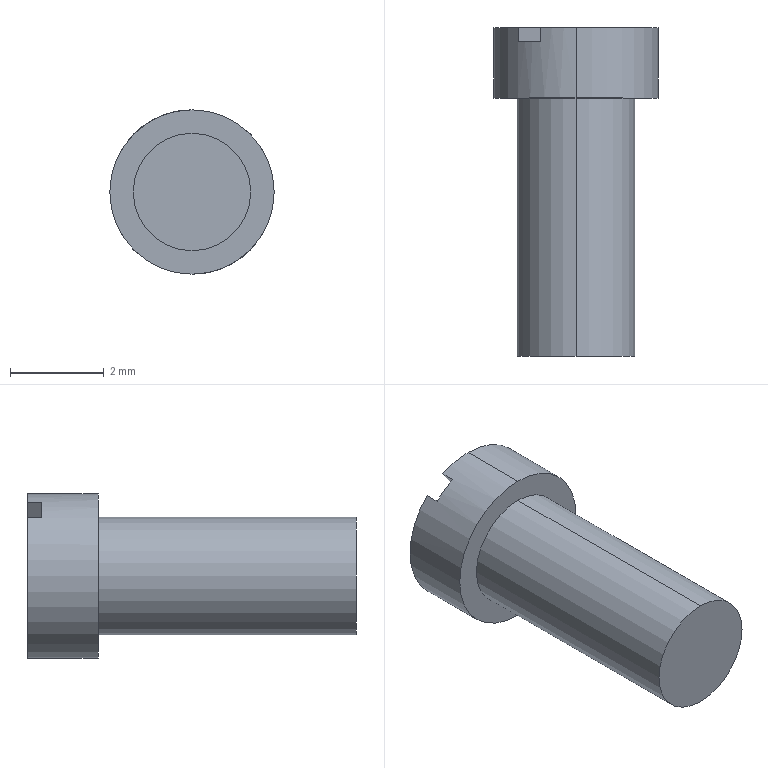Part | SolidWorks | features Cut 1, Extrusion 1, ICE 1 | 1 solid | 11 faces | box 3.5 x 7 x 3.5 mm | volume 40.83 mm3 | plane 7 | cylinder 4 | commonest cylinder face diameters 2.5 x2 3.5 x2
STEP:
#1=CARTESIAN_POINT('',(0.,7.,1.75));
#2=VERTEX_POINT('',#1);
#3=CARTESIAN_POINT('',(1.233,7.,-1.242));
#4=VERTEX_POINT('',#3);
#5=CARTESIAN_POINT('',(0.,7.,0.));
#6=DIRECTION('',(0.,1.,0.));
#7=DIRECTION('',(0.,0.,1.));
#8=AXIS2_PLACEMENT_3D('',#5,#6,#7);
#9=CIRCLE('',#8,1.75);
#10=EDGE_CURVE('',#2,#4,#9,.T.);
#11=ORIENTED_EDGE('',*,*,#10,.F.);
#12=CARTESIAN_POINT('',(0.,5.5,1.75));
#13=VERTEX_POINT('',#12);
#14=CARTESIAN_POINT('',(0.,7.,1.75));
#15=DIRECTION('',(0.,-1.,0.));
#16=VECTOR('',#15,1000.);
#17=LINE('',#14,#16);
#18=EDGE_CURVE('',#2,#13,#17,.T.);
#19=ORIENTED_EDGE('',*,*,#18,.T.);
#20=CARTESIAN_POINT('',(0.,5.5,-1.75));
#21=VERTEX_POINT('',#20);
#22=CARTESIAN_POINT('',(0.,5.5,0.));
#23=DIRECTION('',(0.,1.,0.));
#24=DIRECTION('',(0.,0.,1.));
#25=AXIS2_PLACEMENT_3D('',#22,#23,#24);
#26=CIRCLE('',#25,1.75);
#27=EDGE_CURVE('',#13,#21,#26,.T.);
#28=ORIENTED_EDGE('',*,*,#27,.T.);
#29=CARTESIAN_POINT('',(0.,7.,-1.75));
#30=VERTEX_POINT('',#29);
#31=CARTESIAN_POINT('',(0.,7.,-1.75));
#32=DIRECTION('',(0.,-1.,0.));
#33=VECTOR('',#32,1000.);
#34=LINE('',#31,#33);
#35=EDGE_CURVE('',#30,#21,#34,.T.);
#36=ORIENTED_EDGE('',*,*,#35,.F.);
#37=CARTESIAN_POINT('',(0.7649,7.,-1.574));
#38=VERTEX_POINT('',#37);
#39=CARTESIAN_POINT('',(0.,7.,0.));
#40=DIRECTION('',(0.,1.,0.));
#41=DIRECTION('',(0.,0.,1.));
#42=AXIS2_PLACEMENT_3D('',#39,#40,#41);
#43=CIRCLE('',#42,1.75);
#44=EDGE_CURVE('',#38,#30,#43,.T.);
#45=ORIENTED_EDGE('',*,*,#44,.F.);
#46=CARTESIAN_POINT('',(0.7649,6.7,-1.574));
#47=VERTEX_POINT('',#46);
#48=CARTESIAN_POINT('',(0.7649,7.,-1.574));
#49=DIRECTION('',(0.,-1.,0.));
#50=VECTOR('',#49,1000.);
#51=LINE('',#48,#50);
#52=EDGE_CURVE('',#38,#47,#51,.T.);
#53=ORIENTED_EDGE('',*,*,#52,.T.);
#54=CARTESIAN_POINT('',(1.233,6.7,-1.242));
#55=VERTEX_POINT('',#54);
#56=CARTESIAN_POINT('',(0.,6.7,0.));
#57=DIRECTION('',(0.,1.,0.));
#58=DIRECTION('',(0.,0.,1.));
#59=AXIS2_PLACEMENT_3D('',#56,#57,#58);
#60=CIRCLE('',#59,1.75);
#61=EDGE_CURVE('',#55,#47,#60,.T.);
#62=ORIENTED_EDGE('',*,*,#61,.F.);
#63=CARTESIAN_POINT('',(1.233,7.,-1.242));
#64=DIRECTION('',(0.,1.,0.));
#65=VECTOR('',#64,1000.);
#66=LINE('',#63,#65);
#67=EDGE_CURVE('',#55,#4,#66,.T.);
#68=ORIENTED_EDGE('',*,*,#67,.T.);
#69=EDGE_LOOP('',(#11,#19,#28,#36,#45,#53,#62,#68));
#70=FACE_OUTER_BOUND('',#69,.T.);
#71=CARTESIAN_POINT('',(0.,7.,0.));
#72=DIRECTION('',(0.,-1.,0.));
#73=DIRECTION('',(0.,0.,-1.));
#74=AXIS2_PLACEMENT_3D('',#71,#72,#73);
#75=CYLINDRICAL_SURFACE('',#74,1.75);
#76=ADVANCED_FACE('',(#70),#75,.T.);
#77=CARTESIAN_POINT('',(0.,5.5,1.25));
#78=VERTEX_POINT('',#77);
#79=CARTESIAN_POINT('',(0.,5.5,-1.25));
#80=VERTEX_POINT('',#79);
#81=CARTESIAN_POINT('',(0.,5.5,0.));
#82=DIRECTION('',(0.,1.,0.));
#83=DIRECTION('',(0.,0.,1.));
#84=AXIS2_PLACEMENT_3D('',#81,#82,#83);
#85=CIRCLE('',#84,1.25);
#86=EDGE_CURVE('',#78,#80,#85,.T.);
#87=ORIENTED_EDGE('',*,*,#86,.F.);
#88=CARTESIAN_POINT('',(0.,0.,1.25));
#89=VERTEX_POINT('',#88);
#90=CARTESIAN_POINT('',(0.,5.5,1.25));
#91=DIRECTION('',(0.,-1.,0.));
#92=VECTOR('',#91,1000.);
#93=LINE('',#90,#92);
#94=EDGE_CURVE('',#78,#89,#93,.T.);
#95=ORIENTED_EDGE('',*,*,#94,.T.);
#96=CARTESIAN_POINT('',(0.,0.,-1.25));
#97=VERTEX_POINT('',#96);
#98=CARTESIAN_POINT('',(0.,0.,0.));
#99=DIRECTION('',(0.,1.,0.));
#100=DIRECTION('',(0.,0.,1.));
#101=AXIS2_PLACEMENT_3D('',#98,#99,#100);
#102=CIRCLE('',#101,1.25);
#103=EDGE_CURVE('',#89,#97,#102,.T.);
#104=ORIENTED_EDGE('',*,*,#103,.T.);
#105=CARTESIAN_POINT('',(0.,5.5,-1.25));
#106=DIRECTION('',(0.,-1.,0.));
#107=VECTOR('',#106,1000.);
#108=LINE('',#105,#107);
#109=EDGE_CURVE('',#80,#97,#108,.T.);
#110=ORIENTED_EDGE('',*,*,#109,.F.);
#111=EDGE_LOOP('',(#87,#95,#104,#110));
#112=FACE_OUTER_BOUND('',#111,.T.);
#113=CARTESIAN_POINT('',(0.,5.5,0.));
#114=DIRECTION('',(0.,-1.,0.));
#115=DIRECTION('',(0.,0.,-1.));
#116=AXIS2_PLACEMENT_3D('',#113,#114,#115);
#117=CYLINDRICAL_SURFACE('',#116,1.25);
#118=ADVANCED_FACE('',(#112),#117,.T.);
#119=CARTESIAN_POINT('',(-1.233,7.,1.242));
#120=VERTEX_POINT('',#119);
#121=CARTESIAN_POINT('',(-0.2341,7.,-0.1661));
#122=DIRECTION('',(-0.5787,0.,0.8155));
#123=VECTOR('',#122,1000.);
#124=LINE('',#121,#123);
#125=EDGE_CURVE('',#38,#120,#124,.T.);
#126=ORIENTED_EDGE('',*,*,#125,.F.);
#127=ORIENTED_EDGE('',*,*,#44,.T.);
#128=CARTESIAN_POINT('',(0.,7.,0.));
#129=DIRECTION('',(0.,1.,0.));
#130=DIRECTION('',(0.,0.,1.));
#131=AXIS2_PLACEMENT_3D('',#128,#129,#130);
#132=CIRCLE('',#131,1.75);
#133=EDGE_CURVE('',#30,#120,#132,.T.);
#134=ORIENTED_EDGE('',*,*,#133,.T.);
#135=EDGE_LOOP('',(#126,#127,#134));
#136=FACE_OUTER_BOUND('',#135,.T.);
#137=CARTESIAN_POINT('',(0.,7.,0.));
#138=DIRECTION('',(0.,1.,0.));
#139=DIRECTION('',(0.,0.,1.));
#140=AXIS2_PLACEMENT_3D('',#137,#138,#139);
#141=PLANE('',#140);
#142=ADVANCED_FACE('',(#136),#141,.T.);
#143=ORIENTED_EDGE('',*,*,#94,.F.);
#144=CARTESIAN_POINT('',(0.,5.5,0.));
#145=DIRECTION('',(0.,1.,0.));
#146=DIRECTION('',(0.,0.,1.));
#147=AXIS2_PLACEMENT_3D('',#144,#145,#146);
#148=CIRCLE('',#147,1.25);
#149=EDGE_CURVE('',#80,#78,#148,.T.);
#150=ORIENTED_EDGE('',*,*,#149,.F.);
#151=ORIENTED_EDGE('',*,*,#109,.T.);
#152=CARTESIAN_POINT('',(0.,0.,0.));
#153=DIRECTION('',(0.,1.,0.));
#154=DIRECTION('',(0.,0.,1.));
#155=AXIS2_PLACEMENT_3D('',#152,#153,#154);
#156=CIRCLE('',#155,1.25);
#157=EDGE_CURVE('',#97,#89,#156,.T.);
#158=ORIENTED_EDGE('',*,*,#157,.T.);
#159=EDGE_LOOP('',(#143,#150,#151,#158));
#160=FACE_OUTER_BOUND('',#159,.T.);
#161=CARTESIAN_POINT('',(0.,5.5,0.));
#162=DIRECTION('',(0.,-1.,0.));
#163=DIRECTION('',(0.,0.,-1.));
#164=AXIS2_PLACEMENT_3D('',#161,#162,#163);
#165=CYLINDRICAL_SURFACE('',#164,1.25);
#166=ADVANCED_FACE('',(#160),#165,.T.);
#167=ORIENTED_EDGE('',*,*,#157,.F.);
#168=ORIENTED_EDGE('',*,*,#103,.F.);
#169=EDGE_LOOP('',(#167,#168));
#170=FACE_OUTER_BOUND('',#169,.T.);
#171=CARTESIAN_POINT('',(0.,0.,0.));
#172=DIRECTION('',(0.,1.,0.));
#173=DIRECTION('',(0.,0.,1.));
#174=AXIS2_PLACEMENT_3D('',#171,#172,#173);
#175=PLANE('',#174);
#176=ADVANCED_FACE('',(#170),#175,.F.);
#177=ORIENTED_EDGE('',*,*,#18,.F.);
#178=CARTESIAN_POINT('',(-0.7649,7.,1.574));
#179=VERTEX_POINT('',#178);
#180=CARTESIAN_POINT('',(0.,7.,0.));
#181=DIRECTION('',(0.,1.,0.));
#182=DIRECTION('',(0.,0.,1.));
#183=AXIS2_PLACEMENT_3D('',#180,#181,#182);
#184=CIRCLE('',#183,1.75);
#185=EDGE_CURVE('',#179,#2,#184,.T.);
#186=ORIENTED_EDGE('',*,*,#185,.F.);
#187=CARTESIAN_POINT('',(-0.7649,6.7,1.574));
#188=VERTEX_POINT('',#187);
#189=CARTESIAN_POINT('',(-0.7649,7.,1.574));
#190=DIRECTION('',(0.,-1.,0.));
#191=VECTOR('',#190,1000.);
#192=LINE('',#189,#191);
#193=EDGE_CURVE('',#179,#188,#192,.T.);
#194=ORIENTED_EDGE('',*,*,#193,.T.);
#195=CARTESIAN_POINT('',(-1.233,6.7,1.242));
#196=VERTEX_POINT('',#195);
#197=CARTESIAN_POINT('',(0.,6.7,0.));
#198=DIRECTION('',(0.,1.,0.));
#199=DIRECTION('',(0.,0.,1.));
#200=AXIS2_PLACEMENT_3D('',#197,#198,#199);
#201=CIRCLE('',#200,1.75);
#202=EDGE_CURVE('',#196,#188,#201,.T.);
#203=ORIENTED_EDGE('',*,*,#202,.F.);
#204=CARTESIAN_POINT('',(-1.233,7.,1.242));
#205=DIRECTION('',(0.,1.,0.));
#206=VECTOR('',#205,1000.);
#207=LINE('',#204,#206);
#208=EDGE_CURVE('',#196,#120,#207,.T.);
#209=ORIENTED_EDGE('',*,*,#208,.T.);
#210=ORIENTED_EDGE('',*,*,#133,.F.);
#211=ORIENTED_EDGE('',*,*,#35,.T.);
#212=CARTESIAN_POINT('',(0.,5.5,0.));
#213=DIRECTION('',(0.,1.,0.));
#214=DIRECTION('',(0.,0.,1.));
#215=AXIS2_PLACEMENT_3D('',#212,#213,#214);
#216=CIRCLE('',#215,1.75);
#217=EDGE_CURVE('',#21,#13,#216,.T.);
#218=ORIENTED_EDGE('',*,*,#217,.T.);
#219=EDGE_LOOP('',(#177,#186,#194,#203,#209,#210,#211,#218));
#220=FACE_OUTER_BOUND('',#219,.T.);
#221=CARTESIAN_POINT('',(0.,7.,0.));
#222=DIRECTION('',(0.,-1.,0.));
#223=DIRECTION('',(0.,0.,-1.));
#224=AXIS2_PLACEMENT_3D('',#221,#222,#223);
#225=CYLINDRICAL_SURFACE('',#224,1.75);
#226=ADVANCED_FACE('',(#220),#225,.T.);
#227=CARTESIAN_POINT('',(0.2341,7.,0.1661));
#228=DIRECTION('',(0.5787,0.,-0.8155));
#229=VECTOR('',#228,1000.);
#230=LINE('',#227,#229);
#231=EDGE_CURVE('',#179,#4,#230,.T.);
#232=ORIENTED_EDGE('',*,*,#231,.F.);
#233=ORIENTED_EDGE('',*,*,#185,.T.);
#234=ORIENTED_EDGE('',*,*,#10,.T.);
#235=EDGE_LOOP('',(#232,#233,#234));
#236=FACE_OUTER_BOUND('',#235,.T.);
#237=CARTESIAN_POINT('',(0.,7.,0.));
#238=DIRECTION('',(0.,1.,0.));
#239=DIRECTION('',(0.,0.,1.));
#240=AXIS2_PLACEMENT_3D('',#237,#238,#239);
#241=PLANE('',#240);
#242=ADVANCED_FACE('',(#236),#241,.T.);
#243=ORIENTED_EDGE('',*,*,#149,.T.);
#244=ORIENTED_EDGE('',*,*,#86,.T.);
#245=EDGE_LOOP('',(#243,#244));
#246=FACE_BOUND('',#245,.T.);
#247=ORIENTED_EDGE('',*,*,#217,.F.);
#248=ORIENTED_EDGE('',*,*,#27,.F.);
#249=EDGE_LOOP('',(#247,#248));
#250=FACE_OUTER_BOUND('',#249,.T.);
#251=CARTESIAN_POINT('',(0.,5.5,0.));
#252=DIRECTION('',(0.,1.,0.));
#253=DIRECTION('',(0.,0.,1.));
#254=AXIS2_PLACEMENT_3D('',#251,#252,#253);
#255=PLANE('',#254);
#256=ADVANCED_FACE('',(#246,#250),#255,.F.);
#257=ORIENTED_EDGE('',*,*,#61,.T.);
#258=CARTESIAN_POINT('',(-1.612,6.7,1.775));
#259=DIRECTION('',(-0.5787,0.,0.8155));
#260=VECTOR('',#259,1000.);
#261=LINE('',#258,#260);
#262=EDGE_CURVE('',#47,#196,#261,.T.);
#263=ORIENTED_EDGE('',*,*,#262,.T.);
#264=ORIENTED_EDGE('',*,*,#202,.T.);
#265=CARTESIAN_POINT('',(-1.144,6.7,2.108));
#266=DIRECTION('',(0.5787,0.,-0.8155));
#267=VECTOR('',#266,1000.);
#268=LINE('',#265,#267);
#269=EDGE_CURVE('',#188,#55,#268,.T.);
#270=ORIENTED_EDGE('',*,*,#269,.T.);
#271=EDGE_LOOP('',(#257,#263,#264,#270));
#272=FACE_OUTER_BOUND('',#271,.T.);
#273=CARTESIAN_POINT('',(0.,6.7,0.));
#274=DIRECTION('',(0.,1.,0.));
#275=DIRECTION('',(0.,0.,1.));
#276=AXIS2_PLACEMENT_3D('',#273,#274,#275);
#277=PLANE('',#276);
#278=ADVANCED_FACE('',(#272),#277,.T.);
#279=ORIENTED_EDGE('',*,*,#125,.T.);
#280=ORIENTED_EDGE('',*,*,#208,.F.);
#281=ORIENTED_EDGE('',*,*,#262,.F.);
#282=ORIENTED_EDGE('',*,*,#52,.F.);
#283=EDGE_LOOP('',(#279,#280,#281,#282));
#284=FACE_OUTER_BOUND('',#283,.T.);
#285=CARTESIAN_POINT('',(-1.612,6.7,1.775));
#286=DIRECTION('',(-0.8155,0.,-0.5787));
#287=DIRECTION('',(-0.5787,0.,0.8155));
#288=AXIS2_PLACEMENT_3D('',#285,#286,#287);
#289=PLANE('',#288);
#290=ADVANCED_FACE('',(#284),#289,.F.);
#291=ORIENTED_EDGE('',*,*,#231,.T.);
#292=ORIENTED_EDGE('',*,*,#67,.F.);
#293=ORIENTED_EDGE('',*,*,#269,.F.);
#294=ORIENTED_EDGE('',*,*,#193,.F.);
#295=EDGE_LOOP('',(#291,#292,#293,#294));
#296=FACE_OUTER_BOUND('',#295,.T.);
#297=CARTESIAN_POINT('',(-1.144,6.7,2.108));
#298=DIRECTION('',(0.8155,0.,0.5787));
#299=DIRECTION('',(0.5787,0.,-0.8155));
#300=AXIS2_PLACEMENT_3D('',#297,#298,#299);
#301=PLANE('',#300);
#302=ADVANCED_FACE('',(#296),#301,.F.);
#303=CLOSED_SHELL('',(#76,#118,#142,#166,#176,#226,#242,#256,#278,#290,#302));
#304=MANIFOLD_SOLID_BREP('',#303);
#305=CARTESIAN_POINT('',(0.,0.,0.));
#306=DIRECTION('',(0.,0.,1.));
#307=DIRECTION('',(1.,0.,0.));
#308=AXIS2_PLACEMENT_3D('',#305,#306,#307);
#309=(LENGTH_UNIT()NAMED_UNIT(*)SI_UNIT(.MILLI.,.METRE.));
#310=UNCERTAINTY_MEASURE_WITH_UNIT(LENGTH_MEASURE(0.00001),#309,'','');
#311=(NAMED_UNIT(*)PLANE_ANGLE_UNIT()SI_UNIT($,.RADIAN.));
#312=(NAMED_UNIT(*)SI_UNIT($,.STERADIAN.)SOLID_ANGLE_UNIT());
#313=(GEOMETRIC_REPRESENTATION_CONTEXT(3)GLOBAL_UNCERTAINTY_ASSIGNED_CONTEXT((#310))GLOBAL_UNIT_ASSIGNED_CONTEXT((#309,#311,#312))REPRESENTATION_CONTEXT('',''));
#314=ADVANCED_BREP_SHAPE_REPRESENTATION('',(#304,#308),#313);